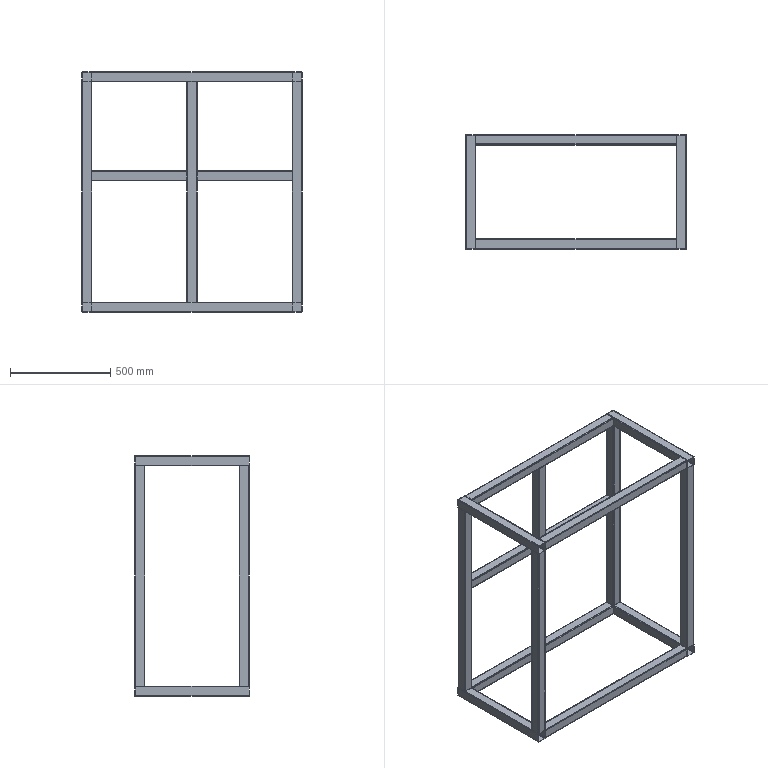Part | SolidWorks | features 3DProfileFeature 1, EndCap 1, WeldMemberFeat 1, WeldmentFeature 1 | 19 solids | 310 faces | box 1100 x 570 x 1200 mm | volume 4774090 mm3 | plane 174 | cylinder 136 | commonest cylinder face diameters 4 x76 8 x60